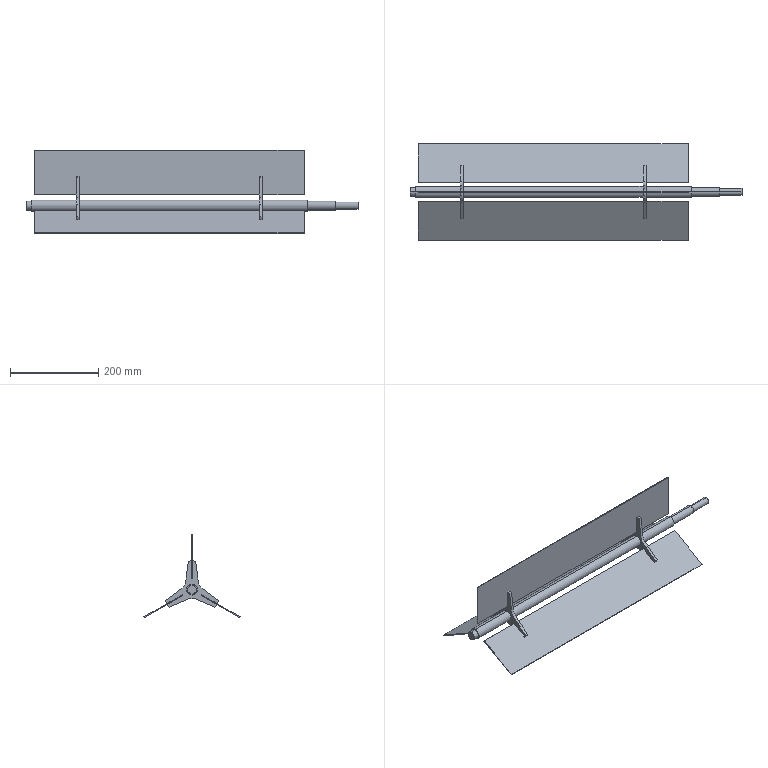Part | SolidWorks | features BaseBody 6, ICE 3 | 6 solids | 87 faces | box 751 x 217.506 x 188.366 mm | volume 750976 mm3 | plane 57 | cylinder 30 | commonest cylinder face diameters 130 x12 25 x6 50 x6 20 x4 16 x2